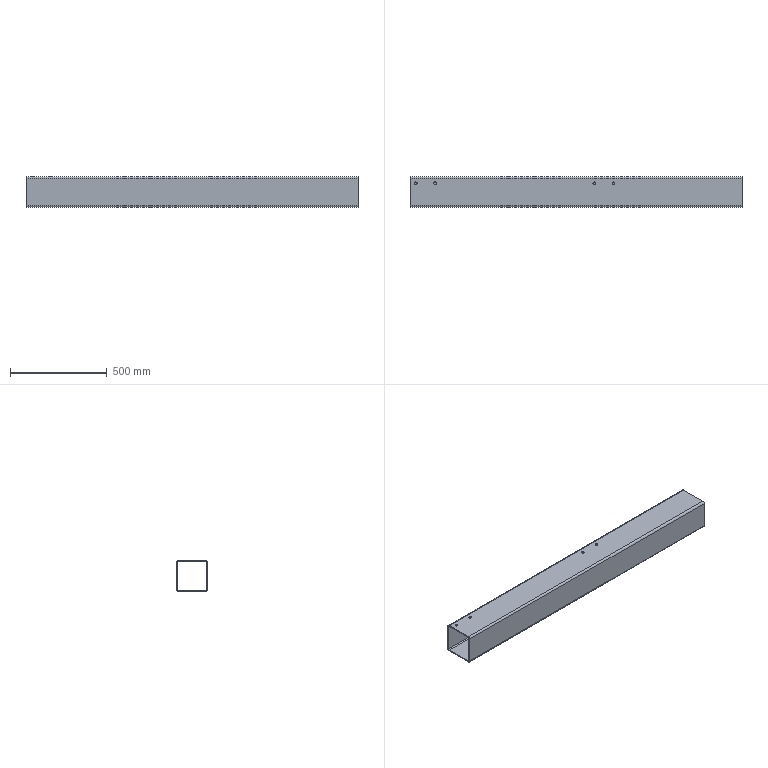Part | SolidWorks | features BaseBody 1 | 1 solid | 26 faces | box 1720 x 160 x 160 mm | volume 5218187 mm3 | cylinder 16 | plane 10 | commonest cylinder face diameters 14 x8 10 x4 20 x4
STEP:
#1=CARTESIAN_POINT('',(-837.,45.,75.));
#2=VERTEX_POINT('',#1);
#3=CARTESIAN_POINT('',(-823.,45.,75.));
#4=VERTEX_POINT('',#3);
#5=CARTESIAN_POINT('',(-830.,45.,75.));
#6=DIRECTION('',(0.,0.,-1.));
#7=DIRECTION('',(0.,1.,0.));
#8=AXIS2_PLACEMENT_3D('',#5,#6,#7);
#9=CIRCLE('',#8,7.);
#10=EDGE_CURVE('',#2,#4,#9,.T.);
#11=ORIENTED_EDGE('',*,*,#10,.T.);
#12=CARTESIAN_POINT('',(-823.,45.,80.));
#13=VERTEX_POINT('',#12);
#14=CARTESIAN_POINT('',(-823.,45.,100.));
#15=DIRECTION('',(0.,0.,1.));
#16=VECTOR('',#15,1000.);
#17=LINE('',#14,#16);
#18=EDGE_CURVE('',#4,#13,#17,.T.);
#19=ORIENTED_EDGE('',*,*,#18,.T.);
#20=CARTESIAN_POINT('',(-837.,45.,80.));
#21=VERTEX_POINT('',#20);
#22=CARTESIAN_POINT('',(-830.,45.,80.));
#23=DIRECTION('',(0.,0.,-1.));
#24=DIRECTION('',(0.,1.,0.));
#25=AXIS2_PLACEMENT_3D('',#22,#23,#24);
#26=CIRCLE('',#25,7.);
#27=EDGE_CURVE('',#21,#13,#26,.T.);
#28=ORIENTED_EDGE('',*,*,#27,.F.);
#29=CARTESIAN_POINT('',(-837.,45.,100.));
#30=DIRECTION('',(0.,0.,1.));
#31=VECTOR('',#30,1000.);
#32=LINE('',#29,#31);
#33=EDGE_CURVE('',#2,#21,#32,.T.);
#34=ORIENTED_EDGE('',*,*,#33,.F.);
#35=EDGE_LOOP('',(#11,#19,#28,#34));
#36=FACE_OUTER_BOUND('',#35,.T.);
#37=CARTESIAN_POINT('',(-830.,45.,100.));
#38=DIRECTION('',(0.,0.,1.));
#39=DIRECTION('',(-1.,0.,0.));
#40=AXIS2_PLACEMENT_3D('',#37,#38,#39);
#41=CYLINDRICAL_SURFACE('',#40,7.);
#42=ADVANCED_FACE('',(#36),#41,.F.);
#43=CARTESIAN_POINT('',(-737.,45.,75.));
#44=VERTEX_POINT('',#43);
#45=CARTESIAN_POINT('',(-723.,45.,75.));
#46=VERTEX_POINT('',#45);
#47=CARTESIAN_POINT('',(-730.,45.,75.));
#48=DIRECTION('',(0.,0.,-1.));
#49=DIRECTION('',(0.,1.,0.));
#50=AXIS2_PLACEMENT_3D('',#47,#48,#49);
#51=CIRCLE('',#50,7.);
#52=EDGE_CURVE('',#44,#46,#51,.T.);
#53=ORIENTED_EDGE('',*,*,#52,.T.);
#54=CARTESIAN_POINT('',(-723.,45.,80.));
#55=VERTEX_POINT('',#54);
#56=CARTESIAN_POINT('',(-723.,45.,100.));
#57=DIRECTION('',(0.,0.,1.));
#58=VECTOR('',#57,1000.);
#59=LINE('',#56,#58);
#60=EDGE_CURVE('',#46,#55,#59,.T.);
#61=ORIENTED_EDGE('',*,*,#60,.T.);
#62=CARTESIAN_POINT('',(-737.,45.,80.));
#63=VERTEX_POINT('',#62);
#64=CARTESIAN_POINT('',(-730.,45.,80.));
#65=DIRECTION('',(0.,0.,-1.));
#66=DIRECTION('',(0.,1.,0.));
#67=AXIS2_PLACEMENT_3D('',#64,#65,#66);
#68=CIRCLE('',#67,7.);
#69=EDGE_CURVE('',#63,#55,#68,.T.);
#70=ORIENTED_EDGE('',*,*,#69,.F.);
#71=CARTESIAN_POINT('',(-737.,45.,100.));
#72=DIRECTION('',(0.,0.,1.));
#73=VECTOR('',#72,1000.);
#74=LINE('',#71,#73);
#75=EDGE_CURVE('',#44,#63,#74,.T.);
#76=ORIENTED_EDGE('',*,*,#75,.F.);
#77=EDGE_LOOP('',(#53,#61,#70,#76));
#78=FACE_OUTER_BOUND('',#77,.T.);
#79=CARTESIAN_POINT('',(-730.,45.,100.));
#80=DIRECTION('',(0.,0.,1.));
#81=DIRECTION('',(-1.,0.,0.));
#82=AXIS2_PLACEMENT_3D('',#79,#80,#81);
#83=CYLINDRICAL_SURFACE('',#82,7.);
#84=ADVANCED_FACE('',(#78),#83,.F.);
#85=CARTESIAN_POINT('',(88.,45.,75.));
#86=VERTEX_POINT('',#85);
#87=CARTESIAN_POINT('',(102.,45.,75.));
#88=VERTEX_POINT('',#87);
#89=CARTESIAN_POINT('',(95.,45.,75.));
#90=DIRECTION('',(0.,0.,-1.));
#91=DIRECTION('',(0.,1.,0.));
#92=AXIS2_PLACEMENT_3D('',#89,#90,#91);
#93=CIRCLE('',#92,7.);
#94=EDGE_CURVE('',#86,#88,#93,.T.);
#95=ORIENTED_EDGE('',*,*,#94,.T.);
#96=CARTESIAN_POINT('',(102.,45.,80.));
#97=VERTEX_POINT('',#96);
#98=CARTESIAN_POINT('',(102.,45.,100.));
#99=DIRECTION('',(0.,0.,1.));
#100=VECTOR('',#99,1000.);
#101=LINE('',#98,#100);
#102=EDGE_CURVE('',#88,#97,#101,.T.);
#103=ORIENTED_EDGE('',*,*,#102,.T.);
#104=CARTESIAN_POINT('',(88.,45.,80.));
#105=VERTEX_POINT('',#104);
#106=CARTESIAN_POINT('',(95.,45.,80.));
#107=DIRECTION('',(0.,0.,-1.));
#108=DIRECTION('',(0.,1.,0.));
#109=AXIS2_PLACEMENT_3D('',#106,#107,#108);
#110=CIRCLE('',#109,7.);
#111=EDGE_CURVE('',#105,#97,#110,.T.);
#112=ORIENTED_EDGE('',*,*,#111,.F.);
#113=CARTESIAN_POINT('',(88.,45.,100.));
#114=DIRECTION('',(0.,0.,1.));
#115=VECTOR('',#114,1000.);
#116=LINE('',#113,#115);
#117=EDGE_CURVE('',#86,#105,#116,.T.);
#118=ORIENTED_EDGE('',*,*,#117,.F.);
#119=EDGE_LOOP('',(#95,#103,#112,#118));
#120=FACE_OUTER_BOUND('',#119,.T.);
#121=CARTESIAN_POINT('',(95.,45.,100.));
#122=DIRECTION('',(0.,0.,1.));
#123=DIRECTION('',(-1.,0.,0.));
#124=AXIS2_PLACEMENT_3D('',#121,#122,#123);
#125=CYLINDRICAL_SURFACE('',#124,7.);
#126=ADVANCED_FACE('',(#120),#125,.F.);
#127=CARTESIAN_POINT('',(188.,45.,75.));
#128=VERTEX_POINT('',#127);
#129=CARTESIAN_POINT('',(202.,45.,75.));
#130=VERTEX_POINT('',#129);
#131=CARTESIAN_POINT('',(195.,45.,75.));
#132=DIRECTION('',(0.,0.,-1.));
#133=DIRECTION('',(0.,1.,0.));
#134=AXIS2_PLACEMENT_3D('',#131,#132,#133);
#135=CIRCLE('',#134,7.);
#136=EDGE_CURVE('',#128,#130,#135,.T.);
#137=ORIENTED_EDGE('',*,*,#136,.T.);
#138=CARTESIAN_POINT('',(202.,45.,80.));
#139=VERTEX_POINT('',#138);
#140=CARTESIAN_POINT('',(202.,45.,100.));
#141=DIRECTION('',(0.,0.,1.));
#142=VECTOR('',#141,1000.);
#143=LINE('',#140,#142);
#144=EDGE_CURVE('',#130,#139,#143,.T.);
#145=ORIENTED_EDGE('',*,*,#144,.T.);
#146=CARTESIAN_POINT('',(188.,45.,80.));
#147=VERTEX_POINT('',#146);
#148=CARTESIAN_POINT('',(195.,45.,80.));
#149=DIRECTION('',(0.,0.,-1.));
#150=DIRECTION('',(0.,1.,0.));
#151=AXIS2_PLACEMENT_3D('',#148,#149,#150);
#152=CIRCLE('',#151,7.);
#153=EDGE_CURVE('',#147,#139,#152,.T.);
#154=ORIENTED_EDGE('',*,*,#153,.F.);
#155=CARTESIAN_POINT('',(188.,45.,100.));
#156=DIRECTION('',(0.,0.,1.));
#157=VECTOR('',#156,1000.);
#158=LINE('',#155,#157);
#159=EDGE_CURVE('',#128,#147,#158,.T.);
#160=ORIENTED_EDGE('',*,*,#159,.F.);
#161=EDGE_LOOP('',(#137,#145,#154,#160));
#162=FACE_OUTER_BOUND('',#161,.T.);
#163=CARTESIAN_POINT('',(195.,45.,100.));
#164=DIRECTION('',(0.,0.,1.));
#165=DIRECTION('',(-1.,0.,0.));
#166=AXIS2_PLACEMENT_3D('',#163,#164,#165);
#167=CYLINDRICAL_SURFACE('',#166,7.);
#168=ADVANCED_FACE('',(#162),#167,.F.);
#169=CARTESIAN_POINT('',(-860.,70.,-80.));
#170=VERTEX_POINT('',#169);
#171=CARTESIAN_POINT('',(-860.,80.,-70.));
#172=VERTEX_POINT('',#171);
#173=CARTESIAN_POINT('',(-860.,70.,-70.));
#174=DIRECTION('',(1.,0.,0.));
#175=DIRECTION('',(0.,0.,-1.));
#176=AXIS2_PLACEMENT_3D('',#173,#174,#175);
#177=CIRCLE('',#176,10.);
#178=EDGE_CURVE('',#170,#172,#177,.T.);
#179=ORIENTED_EDGE('',*,*,#178,.T.);
#180=CARTESIAN_POINT('',(860.,80.,-70.));
#181=VERTEX_POINT('',#180);
#182=CARTESIAN_POINT('',(860.,80.,-70.));
#183=DIRECTION('',(-1.,0.,0.));
#184=VECTOR('',#183,1000.);
#185=LINE('',#182,#184);
#186=EDGE_CURVE('',#181,#172,#185,.T.);
#187=ORIENTED_EDGE('',*,*,#186,.F.);
#188=CARTESIAN_POINT('',(860.,70.,-80.));
#189=VERTEX_POINT('',#188);
#190=CARTESIAN_POINT('',(860.,70.,-70.));
#191=DIRECTION('',(1.,0.,0.));
#192=DIRECTION('',(0.,0.,-1.));
#193=AXIS2_PLACEMENT_3D('',#190,#191,#192);
#194=CIRCLE('',#193,10.);
#195=EDGE_CURVE('',#189,#181,#194,.T.);
#196=ORIENTED_EDGE('',*,*,#195,.F.);
#197=CARTESIAN_POINT('',(860.,70.,-80.));
#198=DIRECTION('',(-1.,0.,0.));
#199=VECTOR('',#198,1000.);
#200=LINE('',#197,#199);
#201=EDGE_CURVE('',#189,#170,#200,.T.);
#202=ORIENTED_EDGE('',*,*,#201,.T.);
#203=EDGE_LOOP('',(#179,#187,#196,#202));
#204=FACE_OUTER_BOUND('',#203,.T.);
#205=CARTESIAN_POINT('',(860.,70.,-70.));
#206=DIRECTION('',(-1.,0.,0.));
#207=DIRECTION('',(0.,0.,1.));
#208=AXIS2_PLACEMENT_3D('',#205,#206,#207);
#209=CYLINDRICAL_SURFACE('',#208,10.);
#210=ADVANCED_FACE('',(#204),#209,.T.);
#211=CARTESIAN_POINT('',(-860.,80.,70.));
#212=VERTEX_POINT('',#211);
#213=CARTESIAN_POINT('',(-860.,80.,-70.));
#214=DIRECTION('',(0.,0.,1.));
#215=VECTOR('',#214,1000.);
#216=LINE('',#213,#215);
#217=EDGE_CURVE('',#172,#212,#216,.T.);
#218=ORIENTED_EDGE('',*,*,#217,.T.);
#219=CARTESIAN_POINT('',(860.,80.,70.));
#220=VERTEX_POINT('',#219);
#221=CARTESIAN_POINT('',(860.,80.,70.));
#222=DIRECTION('',(-1.,0.,0.));
#223=VECTOR('',#222,1000.);
#224=LINE('',#221,#223);
#225=EDGE_CURVE('',#220,#212,#224,.T.);
#226=ORIENTED_EDGE('',*,*,#225,.F.);
#227=CARTESIAN_POINT('',(860.,80.,-70.));
#228=DIRECTION('',(0.,0.,1.));
#229=VECTOR('',#228,1000.);
#230=LINE('',#227,#229);
#231=EDGE_CURVE('',#181,#220,#230,.T.);
#232=ORIENTED_EDGE('',*,*,#231,.F.);
#233=ORIENTED_EDGE('',*,*,#186,.T.);
#234=EDGE_LOOP('',(#218,#226,#232,#233));
#235=FACE_OUTER_BOUND('',#234,.T.);
#236=CARTESIAN_POINT('',(860.,80.,-70.));
#237=DIRECTION('',(0.,-1.,0.));
#238=DIRECTION('',(0.,0.,-1.));
#239=AXIS2_PLACEMENT_3D('',#236,#237,#238);
#240=PLANE('',#239);
#241=ADVANCED_FACE('',(#235),#240,.F.);
#242=CARTESIAN_POINT('',(-860.,70.,80.));
#243=VERTEX_POINT('',#242);
#244=CARTESIAN_POINT('',(-860.,70.,70.));
#245=DIRECTION('',(1.,0.,0.));
#246=DIRECTION('',(0.,0.,-1.));
#247=AXIS2_PLACEMENT_3D('',#244,#245,#246);
#248=CIRCLE('',#247,10.);
#249=EDGE_CURVE('',#212,#243,#248,.T.);
#250=ORIENTED_EDGE('',*,*,#249,.T.);
#251=CARTESIAN_POINT('',(860.,70.,80.));
#252=VERTEX_POINT('',#251);
#253=CARTESIAN_POINT('',(860.,70.,80.));
#254=DIRECTION('',(-1.,0.,0.));
#255=VECTOR('',#254,1000.);
#256=LINE('',#253,#255);
#257=EDGE_CURVE('',#252,#243,#256,.T.);
#258=ORIENTED_EDGE('',*,*,#257,.F.);
#259=CARTESIAN_POINT('',(860.,70.,70.));
#260=DIRECTION('',(1.,0.,0.));
#261=DIRECTION('',(0.,0.,-1.));
#262=AXIS2_PLACEMENT_3D('',#259,#260,#261);
#263=CIRCLE('',#262,10.);
#264=EDGE_CURVE('',#220,#252,#263,.T.);
#265=ORIENTED_EDGE('',*,*,#264,.F.);
#266=ORIENTED_EDGE('',*,*,#225,.T.);
#267=EDGE_LOOP('',(#250,#258,#265,#266));
#268=FACE_OUTER_BOUND('',#267,.T.);
#269=CARTESIAN_POINT('',(860.,70.,70.));
#270=DIRECTION('',(-1.,0.,0.));
#271=DIRECTION('',(0.,0.,1.));
#272=AXIS2_PLACEMENT_3D('',#269,#270,#271);
#273=CYLINDRICAL_SURFACE('',#272,10.);
#274=ADVANCED_FACE('',(#268),#273,.T.);
#275=ORIENTED_EDGE('',*,*,#27,.T.);
#276=CARTESIAN_POINT('',(-830.,45.,80.));
#277=DIRECTION('',(0.,0.,-1.));
#278=DIRECTION('',(0.,1.,0.));
#279=AXIS2_PLACEMENT_3D('',#276,#277,#278);
#280=CIRCLE('',#279,7.);
#281=EDGE_CURVE('',#13,#21,#280,.T.);
#282=ORIENTED_EDGE('',*,*,#281,.T.);
#283=EDGE_LOOP('',(#275,#282));
#284=FACE_BOUND('',#283,.T.);
#285=ORIENTED_EDGE('',*,*,#69,.T.);
#286=CARTESIAN_POINT('',(-730.,45.,80.));
#287=DIRECTION('',(0.,0.,-1.));
#288=DIRECTION('',(0.,1.,0.));
#289=AXIS2_PLACEMENT_3D('',#286,#287,#288);
#290=CIRCLE('',#289,7.);
#291=EDGE_CURVE('',#55,#63,#290,.T.);
#292=ORIENTED_EDGE('',*,*,#291,.T.);
#293=EDGE_LOOP('',(#285,#292));
#294=FACE_BOUND('',#293,.T.);
#295=ORIENTED_EDGE('',*,*,#111,.T.);
#296=CARTESIAN_POINT('',(95.,45.,80.));
#297=DIRECTION('',(0.,0.,-1.));
#298=DIRECTION('',(0.,1.,0.));
#299=AXIS2_PLACEMENT_3D('',#296,#297,#298);
#300=CIRCLE('',#299,7.);
#301=EDGE_CURVE('',#97,#105,#300,.T.);
#302=ORIENTED_EDGE('',*,*,#301,.T.);
#303=EDGE_LOOP('',(#295,#302));
#304=FACE_BOUND('',#303,.T.);
#305=ORIENTED_EDGE('',*,*,#153,.T.);
#306=CARTESIAN_POINT('',(195.,45.,80.));
#307=DIRECTION('',(0.,0.,-1.));
#308=DIRECTION('',(0.,1.,0.));
#309=AXIS2_PLACEMENT_3D('',#306,#307,#308);
#310=CIRCLE('',#309,7.);
#311=EDGE_CURVE('',#139,#147,#310,.T.);
#312=ORIENTED_EDGE('',*,*,#311,.T.);
#313=EDGE_LOOP('',(#305,#312));
#314=FACE_BOUND('',#313,.T.);
#315=CARTESIAN_POINT('',(-860.,-70.,80.));
#316=VERTEX_POINT('',#315);
#317=CARTESIAN_POINT('',(-860.,-70.,80.));
#318=DIRECTION('',(0.,-1.,0.));
#319=VECTOR('',#318,1000.);
#320=LINE('',#317,#319);
#321=EDGE_CURVE('',#243,#316,#320,.T.);
#322=ORIENTED_EDGE('',*,*,#321,.T.);
#323=CARTESIAN_POINT('',(860.,-70.,80.));
#324=VERTEX_POINT('',#323);
#325=CARTESIAN_POINT('',(860.,-70.,80.));
#326=DIRECTION('',(-1.,0.,0.));
#327=VECTOR('',#326,1000.);
#328=LINE('',#325,#327);
#329=EDGE_CURVE('',#324,#316,#328,.T.);
#330=ORIENTED_EDGE('',*,*,#329,.F.);
#331=CARTESIAN_POINT('',(860.,-70.,80.));
#332=DIRECTION('',(0.,-1.,0.));
#333=VECTOR('',#332,1000.);
#334=LINE('',#331,#333);
#335=EDGE_CURVE('',#252,#324,#334,.T.);
#336=ORIENTED_EDGE('',*,*,#335,.F.);
#337=ORIENTED_EDGE('',*,*,#257,.T.);
#338=EDGE_LOOP('',(#322,#330,#336,#337));
#339=FACE_OUTER_BOUND('',#338,.T.);
#340=CARTESIAN_POINT('',(860.,-70.,80.));
#341=DIRECTION('',(0.,0.,-1.));
#342=DIRECTION('',(0.,1.,0.));
#343=AXIS2_PLACEMENT_3D('',#340,#341,#342);
#344=PLANE('',#343);
#345=ADVANCED_FACE('',(#284,#294,#304,#314,#339),#344,.F.);
#346=CARTESIAN_POINT('',(-860.,-80.,70.));
#347=VERTEX_POINT('',#346);
#348=CARTESIAN_POINT('',(-860.,-70.,70.));
#349=DIRECTION('',(1.,0.,0.));
#350=DIRECTION('',(0.,0.,-1.));
#351=AXIS2_PLACEMENT_3D('',#348,#349,#350);
#352=CIRCLE('',#351,10.);
#353=EDGE_CURVE('',#316,#347,#352,.T.);
#354=ORIENTED_EDGE('',*,*,#353,.T.);
#355=CARTESIAN_POINT('',(860.,-80.,70.));
#356=VERTEX_POINT('',#355);
#357=CARTESIAN_POINT('',(860.,-80.,70.));
#358=DIRECTION('',(-1.,0.,0.));
#359=VECTOR('',#358,1000.);
#360=LINE('',#357,#359);
#361=EDGE_CURVE('',#356,#347,#360,.T.);
#362=ORIENTED_EDGE('',*,*,#361,.F.);
#363=CARTESIAN_POINT('',(860.,-70.,70.));
#364=DIRECTION('',(1.,0.,0.));
#365=DIRECTION('',(0.,0.,-1.));
#366=AXIS2_PLACEMENT_3D('',#363,#364,#365);
#367=CIRCLE('',#366,10.);
#368=EDGE_CURVE('',#324,#356,#367,.T.);
#369=ORIENTED_EDGE('',*,*,#368,.F.);
#370=ORIENTED_EDGE('',*,*,#329,.T.);
#371=EDGE_LOOP('',(#354,#362,#369,#370));
#372=FACE_OUTER_BOUND('',#371,.T.);
#373=CARTESIAN_POINT('',(860.,-70.,70.));
#374=DIRECTION('',(-1.,0.,0.));
#375=DIRECTION('',(0.,0.,1.));
#376=AXIS2_PLACEMENT_3D('',#373,#374,#375);
#377=CYLINDRICAL_SURFACE('',#376,10.);
#378=ADVANCED_FACE('',(#372),#377,.T.);
#379=CARTESIAN_POINT('',(-860.,-80.,-70.));
#380=VERTEX_POINT('',#379);
#381=CARTESIAN_POINT('',(-860.,-80.,70.));
#382=DIRECTION('',(0.,0.,-1.));
#383=VECTOR('',#382,1000.);
#384=LINE('',#381,#383);
#385=EDGE_CURVE('',#347,#380,#384,.T.);
#386=ORIENTED_EDGE('',*,*,#385,.T.);
#387=CARTESIAN_POINT('',(860.,-80.,-70.));
#388=VERTEX_POINT('',#387);
#389=CARTESIAN_POINT('',(860.,-80.,-70.));
#390=DIRECTION('',(-1.,0.,0.));
#391=VECTOR('',#390,1000.);
#392=LINE('',#389,#391);
#393=EDGE_CURVE('',#388,#380,#392,.T.);
#394=ORIENTED_EDGE('',*,*,#393,.F.);
#395=CARTESIAN_POINT('',(860.,-80.,70.));
#396=DIRECTION('',(0.,0.,-1.));
#397=VECTOR('',#396,1000.);
#398=LINE('',#395,#397);
#399=EDGE_CURVE('',#356,#388,#398,.T.);
#400=ORIENTED_EDGE('',*,*,#399,.F.);
#401=ORIENTED_EDGE('',*,*,#361,.T.);
#402=EDGE_LOOP('',(#386,#394,#400,#401));
#403=FACE_OUTER_BOUND('',#402,.T.);
#404=CARTESIAN_POINT('',(860.,-80.,70.));
#405=DIRECTION('',(0.,1.,0.));
#406=DIRECTION('',(0.,0.,1.));
#407=AXIS2_PLACEMENT_3D('',#404,#405,#406);
#408=PLANE('',#407);
#409=ADVANCED_FACE('',(#403),#408,.F.);
#410=CARTESIAN_POINT('',(-860.,-70.,-80.));
#411=VERTEX_POINT('',#410);
#412=CARTESIAN_POINT('',(-860.,-70.,-70.));
#413=DIRECTION('',(1.,0.,0.));
#414=DIRECTION('',(0.,0.,-1.));
#415=AXIS2_PLACEMENT_3D('',#412,#413,#414);
#416=CIRCLE('',#415,10.);
#417=EDGE_CURVE('',#380,#411,#416,.T.);
#418=ORIENTED_EDGE('',*,*,#417,.T.);
#419=CARTESIAN_POINT('',(860.,-70.,-80.));
#420=VERTEX_POINT('',#419);
#421=CARTESIAN_POINT('',(860.,-70.,-80.));
#422=DIRECTION('',(-1.,0.,0.));
#423=VECTOR('',#422,1000.);
#424=LINE('',#421,#423);
#425=EDGE_CURVE('',#420,#411,#424,.T.);
#426=ORIENTED_EDGE('',*,*,#425,.F.);
#427=CARTESIAN_POINT('',(860.,-70.,-70.));
#428=DIRECTION('',(1.,0.,0.));
#429=DIRECTION('',(0.,0.,-1.));
#430=AXIS2_PLACEMENT_3D('',#427,#428,#429);
#431=CIRCLE('',#430,10.);
#432=EDGE_CURVE('',#388,#420,#431,.T.);
#433=ORIENTED_EDGE('',*,*,#432,.F.);
#434=ORIENTED_EDGE('',*,*,#393,.T.);
#435=EDGE_LOOP('',(#418,#426,#433,#434));
#436=FACE_OUTER_BOUND('',#435,.T.);
#437=CARTESIAN_POINT('',(860.,-70.,-70.));
#438=DIRECTION('',(-1.,0.,0.));
#439=DIRECTION('',(0.,0.,1.));
#440=AXIS2_PLACEMENT_3D('',#437,#438,#439);
#441=CYLINDRICAL_SURFACE('',#440,10.);
#442=ADVANCED_FACE('',(#436),#441,.T.);
#443=CARTESIAN_POINT('',(-860.,75.,70.));
#444=VERTEX_POINT('',#443);
#445=CARTESIAN_POINT('',(-860.,70.,75.));
#446=VERTEX_POINT('',#445);
#447=CARTESIAN_POINT('',(-860.,70.,70.));
#448=DIRECTION('',(1.,0.,0.));
#449=DIRECTION('',(0.,0.,-1.));
#450=AXIS2_PLACEMENT_3D('',#447,#448,#449);
#451=CIRCLE('',#450,5.);
#452=EDGE_CURVE('',#444,#446,#451,.T.);
#453=ORIENTED_EDGE('',*,*,#452,.F.);
#454=CARTESIAN_POINT('',(860.,75.,70.));
#455=VERTEX_POINT('',#454);
#456=CARTESIAN_POINT('',(860.,75.,70.));
#457=DIRECTION('',(-1.,0.,0.));
#458=VECTOR('',#457,1000.);
#459=LINE('',#456,#458);
#460=EDGE_CURVE('',#455,#444,#459,.T.);
#461=ORIENTED_EDGE('',*,*,#460,.F.);
#462=CARTESIAN_POINT('',(860.,70.,75.));
#463=VERTEX_POINT('',#462);
#464=CARTESIAN_POINT('',(860.,70.,70.));
#465=DIRECTION('',(1.,0.,0.));
#466=DIRECTION('',(0.,0.,-1.));
#467=AXIS2_PLACEMENT_3D('',#464,#465,#466);
#468=CIRCLE('',#467,5.);
#469=EDGE_CURVE('',#455,#463,#468,.T.);
#470=ORIENTED_EDGE('',*,*,#469,.T.);
#471=CARTESIAN_POINT('',(860.,70.,75.));
#472=DIRECTION('',(-1.,0.,0.));
#473=VECTOR('',#472,1000.);
#474=LINE('',#471,#473);
#475=EDGE_CURVE('',#463,#446,#474,.T.);
#476=ORIENTED_EDGE('',*,*,#475,.T.);
#477=EDGE_LOOP('',(#453,#461,#470,#476));
#478=FACE_OUTER_BOUND('',#477,.T.);
#479=CARTESIAN_POINT('',(860.,70.,70.));
#480=DIRECTION('',(-1.,0.,0.));
#481=DIRECTION('',(0.,0.,1.));
#482=AXIS2_PLACEMENT_3D('',#479,#480,#481);
#483=CYLINDRICAL_SURFACE('',#482,5.);
#484=ADVANCED_FACE('',(#478),#483,.F.);
#485=CARTESIAN_POINT('',(-860.,75.,-70.));
#486=VERTEX_POINT('',#485);
#487=CARTESIAN_POINT('',(-860.,75.,-70.));
#488=DIRECTION('',(0.,0.,1.));
#489=VECTOR('',#488,1000.);
#490=LINE('',#487,#489);
#491=EDGE_CURVE('',#486,#444,#490,.T.);
#492=ORIENTED_EDGE('',*,*,#491,.F.);
#493=CARTESIAN_POINT('',(860.,75.,-70.));
#494=VERTEX_POINT('',#493);
#495=CARTESIAN_POINT('',(860.,75.,-70.));
#496=DIRECTION('',(-1.,0.,0.));
#497=VECTOR('',#496,1000.);
#498=LINE('',#495,#497);
#499=EDGE_CURVE('',#494,#486,#498,.T.);
#500=ORIENTED_EDGE('',*,*,#499,.F.);
#501=CARTESIAN_POINT('',(860.,75.,-70.));
#502=DIRECTION('',(0.,0.,1.));
#503=VECTOR('',#502,1000.);
#504=LINE('',#501,#503);
#505=EDGE_CURVE('',#494,#455,#504,.T.);
#506=ORIENTED_EDGE('',*,*,#505,.T.);
#507=ORIENTED_EDGE('',*,*,#460,.T.);
#508=EDGE_LOOP('',(#492,#500,#506,#507));
#509=FACE_OUTER_BOUND('',#508,.T.);
#510=CARTESIAN_POINT('',(860.,75.,-70.));
#511=DIRECTION('',(0.,-1.,0.));
#512=DIRECTION('',(0.,0.,-1.));
#513=AXIS2_PLACEMENT_3D('',#510,#511,#512);
#514=PLANE('',#513);
#515=ADVANCED_FACE('',(#509),#514,.T.);
#516=CARTESIAN_POINT('',(-860.,70.,-75.));
#517=VERTEX_POINT('',#516);
#518=CARTESIAN_POINT('',(-860.,70.,-70.));
#519=DIRECTION('',(1.,0.,0.));
#520=DIRECTION('',(0.,0.,-1.));
#521=AXIS2_PLACEMENT_3D('',#518,#519,#520);
#522=CIRCLE('',#521,5.);
#523=EDGE_CURVE('',#517,#486,#522,.T.);
#524=ORIENTED_EDGE('',*,*,#523,.F.);
#525=CARTESIAN_POINT('',(860.,70.,-75.));
#526=VERTEX_POINT('',#525);
#527=CARTESIAN_POINT('',(860.,70.,-75.));
#528=DIRECTION('',(-1.,0.,0.));
#529=VECTOR('',#528,1000.);
#530=LINE('',#527,#529);
#531=EDGE_CURVE('',#526,#517,#530,.T.);
#532=ORIENTED_EDGE('',*,*,#531,.F.);
#533=CARTESIAN_POINT('',(860.,70.,-70.));
#534=DIRECTION('',(1.,0.,0.));
#535=DIRECTION('',(0.,0.,-1.));
#536=AXIS2_PLACEMENT_3D('',#533,#534,#535);
#537=CIRCLE('',#536,5.);
#538=EDGE_CURVE('',#526,#494,#537,.T.);
#539=ORIENTED_EDGE('',*,*,#538,.T.);
#540=ORIENTED_EDGE('',*,*,#499,.T.);
#541=EDGE_LOOP('',(#524,#532,#539,#540));
#542=FACE_OUTER_BOUND('',#541,.T.);
#543=CARTESIAN_POINT('',(860.,70.,-70.));
#544=DIRECTION('',(-1.,0.,0.));
#545=DIRECTION('',(0.,0.,1.));
#546=AXIS2_PLACEMENT_3D('',#543,#544,#545);
#547=CYLINDRICAL_SURFACE('',#546,5.);
#548=ADVANCED_FACE('',(#542),#547,.F.);
#549=CARTESIAN_POINT('',(-860.,-70.,-75.));
#550=VERTEX_POINT('',#549);
#551=CARTESIAN_POINT('',(-860.,70.,-75.));
#552=DIRECTION('',(0.,1.,0.));
#553=VECTOR('',#552,1000.);
#554=LINE('',#551,#553);
#555=EDGE_CURVE('',#550,#517,#554,.T.);
#556=ORIENTED_EDGE('',*,*,#555,.F.);
#557=CARTESIAN_POINT('',(860.,-70.,-75.));
#558=VERTEX_POINT('',#557);
#559=CARTESIAN_POINT('',(860.,-70.,-75.));
#560=DIRECTION('',(-1.,0.,0.));
#561=VECTOR('',#560,1000.);
#562=LINE('',#559,#561);
#563=EDGE_CURVE('',#558,#550,#562,.T.);
#564=ORIENTED_EDGE('',*,*,#563,.F.);
#565=CARTESIAN_POINT('',(860.,70.,-75.));
#566=DIRECTION('',(0.,1.,0.));
#567=VECTOR('',#566,1000.);
#568=LINE('',#565,#567);
#569=EDGE_CURVE('',#558,#526,#568,.T.);
#570=ORIENTED_EDGE('',*,*,#569,.T.);
#571=ORIENTED_EDGE('',*,*,#531,.T.);
#572=EDGE_LOOP('',(#556,#564,#570,#571));
#573=FACE_OUTER_BOUND('',#572,.T.);
#574=CARTESIAN_POINT('',(860.,70.,-75.));
#575=DIRECTION('',(0.,0.,1.));
#576=DIRECTION('',(1.,0.,0.));
#577=AXIS2_PLACEMENT_3D('',#574,#575,#576);
#578=PLANE('',#577);
#579=ADVANCED_FACE('',(#573),#578,.T.);
#580=CARTESIAN_POINT('',(-860.,-75.,-70.));
#581=VERTEX_POINT('',#580);
#582=CARTESIAN_POINT('',(-860.,-70.,-70.));
#583=DIRECTION('',(1.,0.,0.));
#584=DIRECTION('',(0.,0.,-1.));
#585=AXIS2_PLACEMENT_3D('',#582,#583,#584);
#586=CIRCLE('',#585,5.);
#587=EDGE_CURVE('',#581,#550,#586,.T.);
#588=ORIENTED_EDGE('',*,*,#587,.F.);
#589=CARTESIAN_POINT('',(860.,-75.,-70.));
#590=VERTEX_POINT('',#589);
#591=CARTESIAN_POINT('',(860.,-75.,-70.));
#592=DIRECTION('',(-1.,0.,0.));
#593=VECTOR('',#592,1000.);
#594=LINE('',#591,#593);
#595=EDGE_CURVE('',#590,#581,#594,.T.);
#596=ORIENTED_EDGE('',*,*,#595,.F.);
#597=CARTESIAN_POINT('',(860.,-70.,-70.));
#598=DIRECTION('',(1.,0.,0.));
#599=DIRECTION('',(0.,0.,-1.));
#600=AXIS2_PLACEMENT_3D('',#597,#598,#599);
#601=CIRCLE('',#600,5.);
#602=EDGE_CURVE('',#590,#558,#601,.T.);
#603=ORIENTED_EDGE('',*,*,#602,.T.);
#604=ORIENTED_EDGE('',*,*,#563,.T.);
#605=EDGE_LOOP('',(#588,#596,#603,#604));
#606=FACE_OUTER_BOUND('',#605,.T.);
#607=CARTESIAN_POINT('',(860.,-70.,-70.));
#608=DIRECTION('',(-1.,0.,0.));
#609=DIRECTION('',(0.,0.,1.));
#610=AXIS2_PLACEMENT_3D('',#607,#608,#609);
#611=CYLINDRICAL_SURFACE('',#610,5.);
#612=ADVANCED_FACE('',(#606),#611,.F.);
#613=CARTESIAN_POINT('',(-860.,-75.,70.));
#614=VERTEX_POINT('',#613);
#615=CARTESIAN_POINT('',(-860.,-75.,70.));
#616=DIRECTION('',(0.,0.,-1.));
#617=VECTOR('',#616,1000.);
#618=LINE('',#615,#617);
#619=EDGE_CURVE('',#614,#581,#618,.T.);
#620=ORIENTED_EDGE('',*,*,#619,.F.);
#621=CARTESIAN_POINT('',(860.,-75.,70.));
#622=VERTEX_POINT('',#621);
#623=CARTESIAN_POINT('',(860.,-75.,70.));
#624=DIRECTION('',(-1.,0.,0.));
#625=VECTOR('',#624,1000.);
#626=LINE('',#623,#625);
#627=EDGE_CURVE('',#622,#614,#626,.T.);
#628=ORIENTED_EDGE('',*,*,#627,.F.);
#629=CARTESIAN_POINT('',(860.,-75.,70.));
#630=DIRECTION('',(0.,0.,-1.));
#631=VECTOR('',#630,1000.);
#632=LINE('',#629,#631);
#633=EDGE_CURVE('',#622,#590,#632,.T.);
#634=ORIENTED_EDGE('',*,*,#633,.T.);
#635=ORIENTED_EDGE('',*,*,#595,.T.);
#636=EDGE_LOOP('',(#620,#628,#634,#635));
#637=FACE_OUTER_BOUND('',#636,.T.);
#638=CARTESIAN_POINT('',(860.,-75.,70.));
#639=DIRECTION('',(0.,1.,0.));
#640=DIRECTION('',(0.,0.,1.));
#641=AXIS2_PLACEMENT_3D('',#638,#639,#640);
#642=PLANE('',#641);
#643=ADVANCED_FACE('',(#637),#642,.T.);
#644=CARTESIAN_POINT('',(-860.,-70.,75.));
#645=VERTEX_POINT('',#644);
#646=CARTESIAN_POINT('',(-860.,-70.,70.));
#647=DIRECTION('',(1.,0.,0.));
#648=DIRECTION('',(0.,0.,-1.));
#649=AXIS2_PLACEMENT_3D('',#646,#647,#648);
#650=CIRCLE('',#649,5.);
#651=EDGE_CURVE('',#645,#614,#650,.T.);
#652=ORIENTED_EDGE('',*,*,#651,.F.);
#653=CARTESIAN_POINT('',(860.,-70.,75.));
#654=VERTEX_POINT('',#653);
#655=CARTESIAN_POINT('',(860.,-70.,75.));
#656=DIRECTION('',(-1.,0.,0.));
#657=VECTOR('',#656,1000.);
#658=LINE('',#655,#657);
#659=EDGE_CURVE('',#654,#645,#658,.T.);
#660=ORIENTED_EDGE('',*,*,#659,.F.);
#661=CARTESIAN_POINT('',(860.,-70.,70.));
#662=DIRECTION('',(1.,0.,0.));
#663=DIRECTION('',(0.,0.,-1.));
#664=AXIS2_PLACEMENT_3D('',#661,#662,#663);
#665=CIRCLE('',#664,5.);
#666=EDGE_CURVE('',#654,#622,#665,.T.);
#667=ORIENTED_EDGE('',*,*,#666,.T.);
#668=ORIENTED_EDGE('',*,*,#627,.T.);
#669=EDGE_LOOP('',(#652,#660,#667,#668));
#670=FACE_OUTER_BOUND('',#669,.T.);
#671=CARTESIAN_POINT('',(860.,-70.,70.));
#672=DIRECTION('',(-1.,0.,0.));
#673=DIRECTION('',(0.,0.,1.));
#674=AXIS2_PLACEMENT_3D('',#671,#672,#673);
#675=CYLINDRICAL_SURFACE('',#674,5.);
#676=ADVANCED_FACE('',(#670),#675,.F.);
#677=ORIENTED_EDGE('',*,*,#10,.F.);
#678=CARTESIAN_POINT('',(-830.,45.,75.));
#679=DIRECTION('',(0.,0.,-1.));
#680=DIRECTION('',(0.,1.,0.));
#681=AXIS2_PLACEMENT_3D('',#678,#679,#680);
#682=CIRCLE('',#681,7.);
#683=EDGE_CURVE('',#4,#2,#682,.T.);
#684=ORIENTED_EDGE('',*,*,#683,.F.);
#685=EDGE_LOOP('',(#677,#684));
#686=FACE_BOUND('',#685,.T.);
#687=ORIENTED_EDGE('',*,*,#52,.F.);
#688=CARTESIAN_POINT('',(-730.,45.,75.));
#689=DIRECTION('',(0.,0.,-1.));
#690=DIRECTION('',(0.,1.,0.));
#691=AXIS2_PLACEMENT_3D('',#688,#689,#690);
#692=CIRCLE('',#691,7.);
#693=EDGE_CURVE('',#46,#44,#692,.T.);
#694=ORIENTED_EDGE('',*,*,#693,.F.);
#695=EDGE_LOOP('',(#687,#694));
#696=FACE_BOUND('',#695,.T.);
#697=ORIENTED_EDGE('',*,*,#94,.F.);
#698=CARTESIAN_POINT('',(95.,45.,75.));
#699=DIRECTION('',(0.,0.,-1.));
#700=DIRECTION('',(0.,1.,0.));
#701=AXIS2_PLACEMENT_3D('',#698,#699,#700);
#702=CIRCLE('',#701,7.);
#703=EDGE_CURVE('',#88,#86,#702,.T.);
#704=ORIENTED_EDGE('',*,*,#703,.F.);
#705=EDGE_LOOP('',(#697,#704));
#706=FACE_BOUND('',#705,.T.);
#707=ORIENTED_EDGE('',*,*,#136,.F.);
#708=CARTESIAN_POINT('',(195.,45.,75.));
#709=DIRECTION('',(0.,0.,-1.));
#710=DIRECTION('',(0.,1.,0.));
#711=AXIS2_PLACEMENT_3D('',#708,#709,#710);
#712=CIRCLE('',#711,7.);
#713=EDGE_CURVE('',#130,#128,#712,.T.);
#714=ORIENTED_EDGE('',*,*,#713,.F.);
#715=EDGE_LOOP('',(#707,#714));
#716=FACE_BOUND('',#715,.T.);
#717=CARTESIAN_POINT('',(-860.,-70.,75.));
#718=DIRECTION('',(0.,-1.,0.));
#719=VECTOR('',#718,1000.);
#720=LINE('',#717,#719);
#721=EDGE_CURVE('',#446,#645,#720,.T.);
#722=ORIENTED_EDGE('',*,*,#721,.F.);
#723=ORIENTED_EDGE('',*,*,#475,.F.);
#724=CARTESIAN_POINT('',(860.,-70.,75.));
#725=DIRECTION('',(0.,-1.,0.));
#726=VECTOR('',#725,1000.);
#727=LINE('',#724,#726);
#728=EDGE_CURVE('',#463,#654,#727,.T.);
#729=ORIENTED_EDGE('',*,*,#728,.T.);
#730=ORIENTED_EDGE('',*,*,#659,.T.);
#731=EDGE_LOOP('',(#722,#723,#729,#730));
#732=FACE_OUTER_BOUND('',#731,.T.);
#733=CARTESIAN_POINT('',(860.,-70.,75.));
#734=DIRECTION('',(0.,0.,-1.));
#735=DIRECTION('',(0.,1.,0.));
#736=AXIS2_PLACEMENT_3D('',#733,#734,#735);
#737=PLANE('',#736);
#738=ADVANCED_FACE('',(#686,#696,#706,#716,#732),#737,.T.);
#739=CARTESIAN_POINT('',(-860.,70.,-80.));
#740=DIRECTION('',(0.,1.,0.));
#741=VECTOR('',#740,1000.);
#742=LINE('',#739,#741);
#743=EDGE_CURVE('',#411,#170,#742,.T.);
#744=ORIENTED_EDGE('',*,*,#743,.T.);
#745=ORIENTED_EDGE('',*,*,#201,.F.);
#746=CARTESIAN_POINT('',(860.,70.,-80.));
#747=DIRECTION('',(0.,1.,0.));
#748=VECTOR('',#747,1000.);
#749=LINE('',#746,#748);
#750=EDGE_CURVE('',#420,#189,#749,.T.);
#751=ORIENTED_EDGE('',*,*,#750,.F.);
#752=ORIENTED_EDGE('',*,*,#425,.T.);
#753=EDGE_LOOP('',(#744,#745,#751,#752));
#754=FACE_OUTER_BOUND('',#753,.T.);
#755=CARTESIAN_POINT('',(860.,70.,-80.));
#756=DIRECTION('',(0.,0.,1.));
#757=DIRECTION('',(1.,0.,0.));
#758=AXIS2_PLACEMENT_3D('',#755,#756,#757);
#759=PLANE('',#758);
#760=ADVANCED_FACE('',(#754),#759,.F.);
#761=ORIENTED_EDGE('',*,*,#469,.F.);
#762=ORIENTED_EDGE('',*,*,#505,.F.);
#763=ORIENTED_EDGE('',*,*,#538,.F.);
#764=ORIENTED_EDGE('',*,*,#569,.F.);
#765=ORIENTED_EDGE('',*,*,#602,.F.);
#766=ORIENTED_EDGE('',*,*,#633,.F.);
#767=ORIENTED_EDGE('',*,*,#666,.F.);
#768=ORIENTED_EDGE('',*,*,#728,.F.);
#769=EDGE_LOOP('',(#761,#762,#763,#764,#765,#766,#767,#768));
#770=FACE_BOUND('',#769,.T.);
#771=ORIENTED_EDGE('',*,*,#195,.T.);
#772=ORIENTED_EDGE('',*,*,#231,.T.);
#773=ORIENTED_EDGE('',*,*,#264,.T.);
#774=ORIENTED_EDGE('',*,*,#335,.T.);
#775=ORIENTED_EDGE('',*,*,#368,.T.);
#776=ORIENTED_EDGE('',*,*,#399,.T.);
#777=ORIENTED_EDGE('',*,*,#432,.T.);
#778=ORIENTED_EDGE('',*,*,#750,.T.);
#779=EDGE_LOOP('',(#771,#772,#773,#774,#775,#776,#777,#778));
#780=FACE_OUTER_BOUND('',#779,.T.);
#781=CARTESIAN_POINT('',(860.,70.,-70.));
#782=DIRECTION('',(1.,0.,0.));
#783=DIRECTION('',(0.,0.,-1.));
#784=AXIS2_PLACEMENT_3D('',#781,#782,#783);
#785=PLANE('',#784);
#786=ADVANCED_FACE('',(#770,#780),#785,.T.);
#787=ORIENTED_EDGE('',*,*,#452,.T.);
#788=ORIENTED_EDGE('',*,*,#721,.T.);
#789=ORIENTED_EDGE('',*,*,#651,.T.);
#790=ORIENTED_EDGE('',*,*,#619,.T.);
#791=ORIENTED_EDGE('',*,*,#587,.T.);
#792=ORIENTED_EDGE('',*,*,#555,.T.);
#793=ORIENTED_EDGE('',*,*,#523,.T.);
#794=ORIENTED_EDGE('',*,*,#491,.T.);
#795=EDGE_LOOP('',(#787,#788,#789,#790,#791,#792,#793,#794));
#796=FACE_BOUND('',#795,.T.);
#797=ORIENTED_EDGE('',*,*,#178,.F.);
#798=ORIENTED_EDGE('',*,*,#743,.F.);
#799=ORIENTED_EDGE('',*,*,#417,.F.);
#800=ORIENTED_EDGE('',*,*,#385,.F.);
#801=ORIENTED_EDGE('',*,*,#353,.F.);
#802=ORIENTED_EDGE('',*,*,#321,.F.);
#803=ORIENTED_EDGE('',*,*,#249,.F.);
#804=ORIENTED_EDGE('',*,*,#217,.F.);
#805=EDGE_LOOP('',(#797,#798,#799,#800,#801,#802,#803,#804));
#806=FACE_OUTER_BOUND('',#805,.T.);
#807=CARTESIAN_POINT('',(-860.,70.,-70.));
#808=DIRECTION('',(1.,0.,0.));
#809=DIRECTION('',(0.,0.,-1.));
#810=AXIS2_PLACEMENT_3D('',#807,#808,#809);
#811=PLANE('',#810);
#812=ADVANCED_FACE('',(#796,#806),#811,.F.);
#813=ORIENTED_EDGE('',*,*,#144,.F.);
#814=ORIENTED_EDGE('',*,*,#713,.T.);
#815=ORIENTED_EDGE('',*,*,#159,.T.);
#816=ORIENTED_EDGE('',*,*,#311,.F.);
#817=EDGE_LOOP('',(#813,#814,#815,#816));
#818=FACE_OUTER_BOUND('',#817,.T.);
#819=CARTESIAN_POINT('',(195.,45.,100.));
#820=DIRECTION('',(0.,0.,1.));
#821=DIRECTION('',(-1.,0.,0.));
#822=AXIS2_PLACEMENT_3D('',#819,#820,#821);
#823=CYLINDRICAL_SURFACE('',#822,7.);
#824=ADVANCED_FACE('',(#818),#823,.F.);
#825=ORIENTED_EDGE('',*,*,#102,.F.);
#826=ORIENTED_EDGE('',*,*,#703,.T.);
#827=ORIENTED_EDGE('',*,*,#117,.T.);
#828=ORIENTED_EDGE('',*,*,#301,.F.);
#829=EDGE_LOOP('',(#825,#826,#827,#828));
#830=FACE_OUTER_BOUND('',#829,.T.);
#831=CARTESIAN_POINT('',(95.,45.,100.));
#832=DIRECTION('',(0.,0.,1.));
#833=DIRECTION('',(-1.,0.,0.));
#834=AXIS2_PLACEMENT_3D('',#831,#832,#833);
#835=CYLINDRICAL_SURFACE('',#834,7.);
#836=ADVANCED_FACE('',(#830),#835,.F.);
#837=ORIENTED_EDGE('',*,*,#60,.F.);
#838=ORIENTED_EDGE('',*,*,#693,.T.);
#839=ORIENTED_EDGE('',*,*,#75,.T.);
#840=ORIENTED_EDGE('',*,*,#291,.F.);
#841=EDGE_LOOP('',(#837,#838,#839,#840));
#842=FACE_OUTER_BOUND('',#841,.T.);
#843=CARTESIAN_POINT('',(-730.,45.,100.));
#844=DIRECTION('',(0.,0.,1.));
#845=DIRECTION('',(-1.,0.,0.));
#846=AXIS2_PLACEMENT_3D('',#843,#844,#845);
#847=CYLINDRICAL_SURFACE('',#846,7.);
#848=ADVANCED_FACE('',(#842),#847,.F.);
#849=ORIENTED_EDGE('',*,*,#18,.F.);
#850=ORIENTED_EDGE('',*,*,#683,.T.);
#851=ORIENTED_EDGE('',*,*,#33,.T.);
#852=ORIENTED_EDGE('',*,*,#281,.F.);
#853=EDGE_LOOP('',(#849,#850,#851,#852));
#854=FACE_OUTER_BOUND('',#853,.T.);
#855=CARTESIAN_POINT('',(-830.,45.,100.));
#856=DIRECTION('',(0.,0.,1.));
#857=DIRECTION('',(-1.,0.,0.));
#858=AXIS2_PLACEMENT_3D('',#855,#856,#857);
#859=CYLINDRICAL_SURFACE('',#858,7.);
#860=ADVANCED_FACE('',(#854),#859,.F.);
#861=CLOSED_SHELL('',(#42,#84,#126,#168,#210,#241,#274,#345,#378,#409,#442,#484,#515,#548,#579,#612,#643,#676,#738,#760,#786,#812,#824,#836,#848,#860));
#862=MANIFOLD_SOLID_BREP('',#861);
#863=CARTESIAN_POINT('',(0.,0.,0.));
#864=DIRECTION('',(0.,0.,1.));
#865=DIRECTION('',(1.,0.,0.));
#866=AXIS2_PLACEMENT_3D('',#863,#864,#865);
#867=(LENGTH_UNIT()NAMED_UNIT(*)SI_UNIT(.MILLI.,.METRE.));
#868=UNCERTAINTY_MEASURE_WITH_UNIT(LENGTH_MEASURE(0.00001),#867,'','');
#869=(NAMED_UNIT(*)PLANE_ANGLE_UNIT()SI_UNIT($,.RADIAN.));
#870=(NAMED_UNIT(*)SI_UNIT($,.STERADIAN.)SOLID_ANGLE_UNIT());
#871=(GEOMETRIC_REPRESENTATION_CONTEXT(3)GLOBAL_UNCERTAINTY_ASSIGNED_CONTEXT((#868))GLOBAL_UNIT_ASSIGNED_CONTEXT((#867,#869,#870))REPRESENTATION_CONTEXT('',''));
#872=ADVANCED_BREP_SHAPE_REPRESENTATION('',(#862,#866),#871);